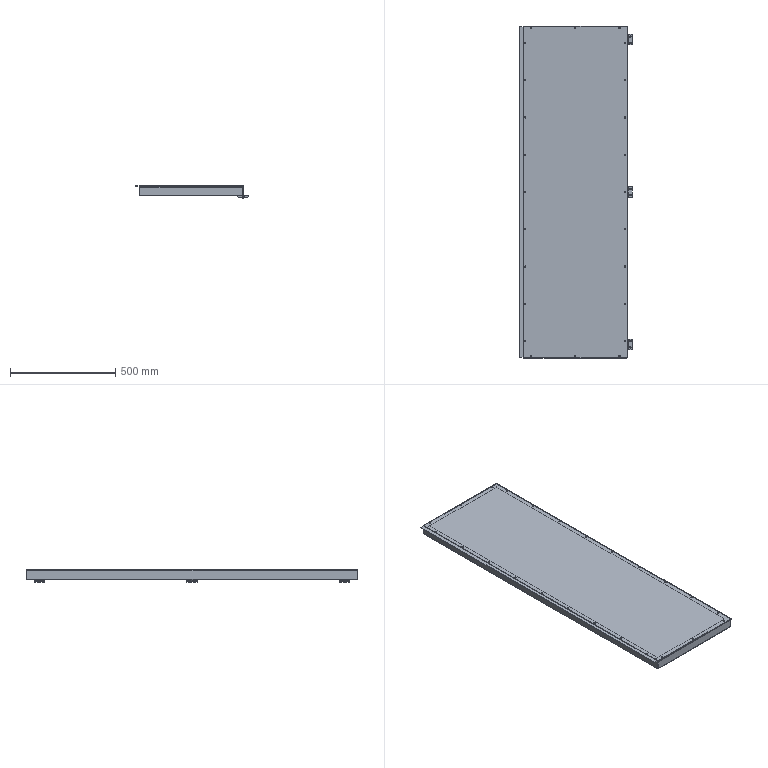Part | SolidWorks | 9 solids | 406 faces | box 537 x 1578 x 59.5 mm | volume 4243510 mm3 | cylinder 196 | plane 174 | cone 24 | spline 12 | commonest cylinder face diameters 5 x60 6.5 x48 6 x24 6.3 x24 12 x24 1.473 x8